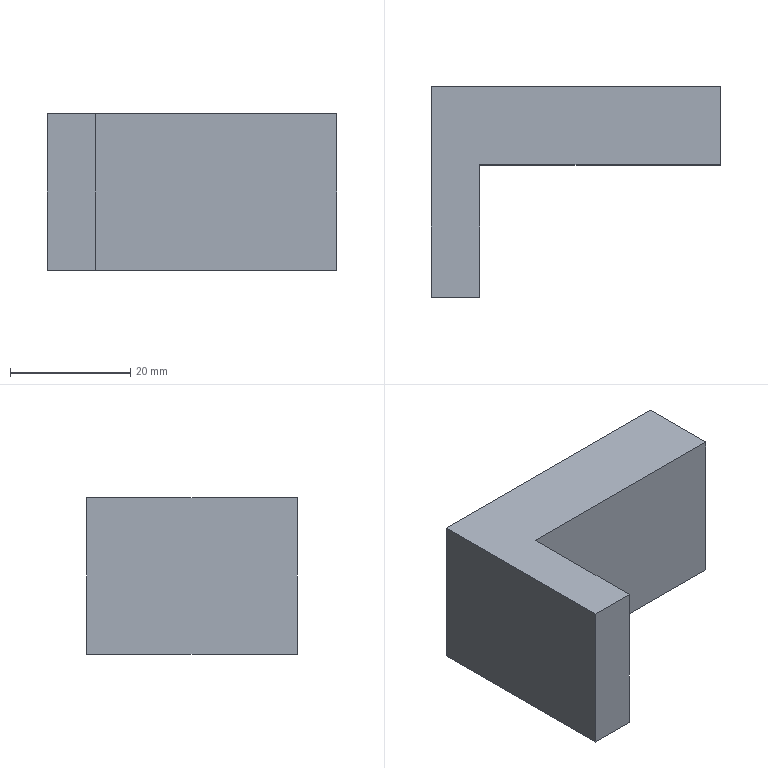Part | STEP file | 001-004-Feeding mechanism slider connecting plate | 1 solid | 8 faces | box 48 x 35 x 26 mm | volume 20800 mm3 | plane 8
STEP:
#1=CARTESIAN_POINT('',(0.,0.,0.));
#2=DIRECTION('',(0.,0.,1.));
#3=DIRECTION('',(1.,0.,0.));
#4=AXIS2_PLACEMENT_3D('',#1,#2,#3);
#5=CARTESIAN_POINT('',(24.,4.5,26.));
#6=VERTEX_POINT('',#5);
#7=CARTESIAN_POINT('',(24.,17.5,26.));
#8=VERTEX_POINT('',#7);
#9=CARTESIAN_POINT('',(24.,-17.5,26.));
#10=DIRECTION('',(0.,1.,0.));
#11=VECTOR('',#10,1.);
#12=LINE('',#9,#11);
#13=CARTESIAN_POINT('',(24.,-17.5,26.));
#14=DIRECTION('',(-1.,0.,0.));
#15=DIRECTION('',(0.,0.,1.));
#16=AXIS2_PLACEMENT_3D('',#13,#14,#15);
#17=PLANE('',#16);
#18=CARTESIAN_POINT('',(0.,0.));
#19=DIRECTION('',(0.,1.));
#20=VECTOR('',#19,1.);
#21=LINE('',#18,#20);
#22=(GEOMETRIC_REPRESENTATION_CONTEXT(2)PARAMETRIC_REPRESENTATION_CONTEXT()REPRESENTATION_CONTEXT('',''));
#23=DEFINITIONAL_REPRESENTATION('',(#21),#22);
#24=PCURVE('',#17,#23);
#25=CARTESIAN_POINT('',(0.,0.,26.));
#26=DIRECTION('',(0.,0.,-1.));
#27=DIRECTION('',(-1.,0.,0.));
#28=AXIS2_PLACEMENT_3D('',#25,#26,#27);
#29=PLANE('',#28);
#30=CARTESIAN_POINT('',(-24.,-17.5));
#31=DIRECTION('',(0.,1.));
#32=VECTOR('',#31,1.);
#33=LINE('',#30,#32);
#34=(GEOMETRIC_REPRESENTATION_CONTEXT(2)PARAMETRIC_REPRESENTATION_CONTEXT()REPRESENTATION_CONTEXT('',''));
#35=DEFINITIONAL_REPRESENTATION('',(#33),#34);
#36=PCURVE('',#29,#35);
#37=SURFACE_CURVE('',#12,(#24,#36),.PCURVE_S1.);
#38=EDGE_CURVE('',#6,#8,#37,.T.);
#39=ORIENTED_EDGE('',*,*,#38,.F.);
#40=CARTESIAN_POINT('',(24.,4.5,0.));
#41=VERTEX_POINT('',#40);
#42=CARTESIAN_POINT('',(24.,4.5,0.));
#43=DIRECTION('',(0.,0.,1.));
#44=VECTOR('',#43,1.);
#45=LINE('',#42,#44);
#46=CARTESIAN_POINT('',(-26.,22.));
#47=DIRECTION('',(1.,0.));
#48=VECTOR('',#47,1.);
#49=LINE('',#46,#48);
#50=(GEOMETRIC_REPRESENTATION_CONTEXT(2)PARAMETRIC_REPRESENTATION_CONTEXT()REPRESENTATION_CONTEXT('',''));
#51=DEFINITIONAL_REPRESENTATION('',(#49),#50);
#52=PCURVE('',#17,#51);
#53=CARTESIAN_POINT('',(24.,4.5,0.));
#54=DIRECTION('',(0.,1.,0.));
#55=DIRECTION('',(-1.,0.,0.));
#56=AXIS2_PLACEMENT_3D('',#53,#54,#55);
#57=PLANE('',#56);
#58=CARTESIAN_POINT('',(0.,0.));
#59=DIRECTION('',(0.,1.));
#60=VECTOR('',#59,1.);
#61=LINE('',#58,#60);
#62=(GEOMETRIC_REPRESENTATION_CONTEXT(2)PARAMETRIC_REPRESENTATION_CONTEXT()REPRESENTATION_CONTEXT('',''));
#63=DEFINITIONAL_REPRESENTATION('',(#61),#62);
#64=PCURVE('',#57,#63);
#65=SURFACE_CURVE('',#45,(#52,#64),.PCURVE_S1.);
#66=EDGE_CURVE('',#41,#6,#65,.T.);
#67=ORIENTED_EDGE('',*,*,#66,.F.);
#68=CARTESIAN_POINT('',(24.,17.5,0.));
#69=VERTEX_POINT('',#68);
#70=CARTESIAN_POINT('',(24.,-17.5,0.));
#71=DIRECTION('',(0.,1.,0.));
#72=VECTOR('',#71,1.);
#73=LINE('',#70,#72);
#74=CARTESIAN_POINT('',(-26.,0.));
#75=DIRECTION('',(0.,1.));
#76=VECTOR('',#75,1.);
#77=LINE('',#74,#76);
#78=(GEOMETRIC_REPRESENTATION_CONTEXT(2)PARAMETRIC_REPRESENTATION_CONTEXT()REPRESENTATION_CONTEXT('',''));
#79=DEFINITIONAL_REPRESENTATION('',(#77),#78);
#80=PCURVE('',#17,#79);
#81=CARTESIAN_POINT('',(0.,0.,0.));
#82=DIRECTION('',(0.,0.,-1.));
#83=DIRECTION('',(-1.,0.,0.));
#84=AXIS2_PLACEMENT_3D('',#81,#82,#83);
#85=PLANE('',#84);
#86=CARTESIAN_POINT('',(-24.,-17.5));
#87=DIRECTION('',(0.,1.));
#88=VECTOR('',#87,1.);
#89=LINE('',#86,#88);
#90=(GEOMETRIC_REPRESENTATION_CONTEXT(2)PARAMETRIC_REPRESENTATION_CONTEXT()REPRESENTATION_CONTEXT('',''));
#91=DEFINITIONAL_REPRESENTATION('',(#89),#90);
#92=PCURVE('',#85,#91);
#93=SURFACE_CURVE('',#73,(#80,#92),.PCURVE_S1.);
#94=EDGE_CURVE('',#41,#69,#93,.T.);
#95=ORIENTED_EDGE('',*,*,#94,.T.);
#96=CARTESIAN_POINT('',(24.,17.5,26.));
#97=DIRECTION('',(0.,0.,-1.));
#98=VECTOR('',#97,1.);
#99=LINE('',#96,#98);
#100=CARTESIAN_POINT('',(0.,35.));
#101=DIRECTION('',(-1.,0.));
#102=VECTOR('',#101,1.);
#103=LINE('',#100,#102);
#104=(GEOMETRIC_REPRESENTATION_CONTEXT(2)PARAMETRIC_REPRESENTATION_CONTEXT()REPRESENTATION_CONTEXT('',''));
#105=DEFINITIONAL_REPRESENTATION('',(#103),#104);
#106=PCURVE('',#17,#105);
#107=CARTESIAN_POINT('',(-24.,17.5,26.));
#108=DIRECTION('',(0.,-1.,0.));
#109=DIRECTION('',(0.,0.,-1.));
#110=AXIS2_PLACEMENT_3D('',#107,#108,#109);
#111=PLANE('',#110);
#112=CARTESIAN_POINT('',(0.,48.));
#113=DIRECTION('',(1.,0.));
#114=VECTOR('',#113,1.);
#115=LINE('',#112,#114);
#116=(GEOMETRIC_REPRESENTATION_CONTEXT(2)PARAMETRIC_REPRESENTATION_CONTEXT()REPRESENTATION_CONTEXT('',''));
#117=DEFINITIONAL_REPRESENTATION('',(#115),#116);
#118=PCURVE('',#111,#117);
#119=SURFACE_CURVE('',#99,(#106,#118),.PCURVE_S1.);
#120=EDGE_CURVE('',#8,#69,#119,.T.);
#121=ORIENTED_EDGE('',*,*,#120,.F.);
#122=EDGE_LOOP('',(#39,#67,#95,#121));
#123=FACE_BOUND('',#122,.T.);
#124=ADVANCED_FACE('',(#123),#17,.F.);
#125=CARTESIAN_POINT('',(-24.,17.5,0.));
#126=VERTEX_POINT('',#125);
#127=CARTESIAN_POINT('',(-24.,17.5,0.));
#128=DIRECTION('',(-1.,0.,0.));
#129=VECTOR('',#128,1.);
#130=LINE('',#127,#129);
#131=CARTESIAN_POINT('',(26.,0.));
#132=DIRECTION('',(0.,-1.));
#133=VECTOR('',#132,1.);
#134=LINE('',#131,#133);
#135=(GEOMETRIC_REPRESENTATION_CONTEXT(2)PARAMETRIC_REPRESENTATION_CONTEXT()REPRESENTATION_CONTEXT('',''));
#136=DEFINITIONAL_REPRESENTATION('',(#134),#135);
#137=PCURVE('',#111,#136);
#138=CARTESIAN_POINT('',(24.,17.5));
#139=DIRECTION('',(1.,0.));
#140=VECTOR('',#139,1.);
#141=LINE('',#138,#140);
#142=(GEOMETRIC_REPRESENTATION_CONTEXT(2)PARAMETRIC_REPRESENTATION_CONTEXT()REPRESENTATION_CONTEXT('',''));
#143=DEFINITIONAL_REPRESENTATION('',(#141),#142);
#144=PCURVE('',#85,#143);
#145=SURFACE_CURVE('',#130,(#137,#144),.PCURVE_S1.);
#146=EDGE_CURVE('',#69,#126,#145,.T.);
#147=ORIENTED_EDGE('',*,*,#146,.T.);
#148=CARTESIAN_POINT('',(-24.,17.5,26.));
#149=VERTEX_POINT('',#148);
#150=CARTESIAN_POINT('',(-24.,17.5,26.));
#151=DIRECTION('',(0.,0.,-1.));
#152=VECTOR('',#151,1.);
#153=LINE('',#150,#152);
#154=CARTESIAN_POINT('',(0.,0.));
#155=DIRECTION('',(1.,0.));
#156=VECTOR('',#155,1.);
#157=LINE('',#154,#156);
#158=(GEOMETRIC_REPRESENTATION_CONTEXT(2)PARAMETRIC_REPRESENTATION_CONTEXT()REPRESENTATION_CONTEXT('',''));
#159=DEFINITIONAL_REPRESENTATION('',(#157),#158);
#160=PCURVE('',#111,#159);
#161=CARTESIAN_POINT('',(-24.,-17.5,26.));
#162=DIRECTION('',(1.,0.,0.));
#163=DIRECTION('',(0.,0.,-1.));
#164=AXIS2_PLACEMENT_3D('',#161,#162,#163);
#165=PLANE('',#164);
#166=CARTESIAN_POINT('',(0.,35.));
#167=DIRECTION('',(1.,0.));
#168=VECTOR('',#167,1.);
#169=LINE('',#166,#168);
#170=(GEOMETRIC_REPRESENTATION_CONTEXT(2)PARAMETRIC_REPRESENTATION_CONTEXT()REPRESENTATION_CONTEXT('',''));
#171=DEFINITIONAL_REPRESENTATION('',(#169),#170);
#172=PCURVE('',#165,#171);
#173=SURFACE_CURVE('',#153,(#160,#172),.PCURVE_S1.);
#174=EDGE_CURVE('',#149,#126,#173,.T.);
#175=ORIENTED_EDGE('',*,*,#174,.F.);
#176=CARTESIAN_POINT('',(-24.,17.5,26.));
#177=DIRECTION('',(-1.,0.,0.));
#178=VECTOR('',#177,1.);
#179=LINE('',#176,#178);
#180=CARTESIAN_POINT('',(0.,0.));
#181=DIRECTION('',(0.,-1.));
#182=VECTOR('',#181,1.);
#183=LINE('',#180,#182);
#184=(GEOMETRIC_REPRESENTATION_CONTEXT(2)PARAMETRIC_REPRESENTATION_CONTEXT()REPRESENTATION_CONTEXT('',''));
#185=DEFINITIONAL_REPRESENTATION('',(#183),#184);
#186=PCURVE('',#111,#185);
#187=CARTESIAN_POINT('',(24.,17.5));
#188=DIRECTION('',(1.,0.));
#189=VECTOR('',#188,1.);
#190=LINE('',#187,#189);
#191=(GEOMETRIC_REPRESENTATION_CONTEXT(2)PARAMETRIC_REPRESENTATION_CONTEXT()REPRESENTATION_CONTEXT('',''));
#192=DEFINITIONAL_REPRESENTATION('',(#190),#191);
#193=PCURVE('',#29,#192);
#194=SURFACE_CURVE('',#179,(#186,#193),.PCURVE_S1.);
#195=EDGE_CURVE('',#8,#149,#194,.T.);
#196=ORIENTED_EDGE('',*,*,#195,.F.);
#197=ORIENTED_EDGE('',*,*,#120,.T.);
#198=EDGE_LOOP('',(#147,#175,#196,#197));
#199=FACE_BOUND('',#198,.T.);
#200=ADVANCED_FACE('',(#199),#111,.F.);
#201=CARTESIAN_POINT('',(-24.,-17.5,0.));
#202=VERTEX_POINT('',#201);
#203=CARTESIAN_POINT('',(-24.,-17.5,0.));
#204=DIRECTION('',(0.,-1.,0.));
#205=VECTOR('',#204,1.);
#206=LINE('',#203,#205);
#207=CARTESIAN_POINT('',(26.,0.));
#208=DIRECTION('',(0.,-1.));
#209=VECTOR('',#208,1.);
#210=LINE('',#207,#209);
#211=(GEOMETRIC_REPRESENTATION_CONTEXT(2)PARAMETRIC_REPRESENTATION_CONTEXT()REPRESENTATION_CONTEXT('',''));
#212=DEFINITIONAL_REPRESENTATION('',(#210),#211);
#213=PCURVE('',#165,#212);
#214=CARTESIAN_POINT('',(24.,-17.5));
#215=DIRECTION('',(0.,-1.));
#216=VECTOR('',#215,1.);
#217=LINE('',#214,#216);
#218=(GEOMETRIC_REPRESENTATION_CONTEXT(2)PARAMETRIC_REPRESENTATION_CONTEXT()REPRESENTATION_CONTEXT('',''));
#219=DEFINITIONAL_REPRESENTATION('',(#217),#218);
#220=PCURVE('',#85,#219);
#221=SURFACE_CURVE('',#206,(#213,#220),.PCURVE_S1.);
#222=EDGE_CURVE('',#126,#202,#221,.T.);
#223=ORIENTED_EDGE('',*,*,#222,.T.);
#224=CARTESIAN_POINT('',(-24.,-17.5,26.));
#225=VERTEX_POINT('',#224);
#226=CARTESIAN_POINT('',(-24.,-17.5,26.));
#227=DIRECTION('',(0.,0.,-1.));
#228=VECTOR('',#227,1.);
#229=LINE('',#226,#228);
#230=CARTESIAN_POINT('',(0.,0.));
#231=DIRECTION('',(1.,0.));
#232=VECTOR('',#231,1.);
#233=LINE('',#230,#232);
#234=(GEOMETRIC_REPRESENTATION_CONTEXT(2)PARAMETRIC_REPRESENTATION_CONTEXT()REPRESENTATION_CONTEXT('',''));
#235=DEFINITIONAL_REPRESENTATION('',(#233),#234);
#236=PCURVE('',#165,#235);
#237=CARTESIAN_POINT('',(-24.,-17.5,26.));
#238=DIRECTION('',(0.,1.,0.));
#239=DIRECTION('',(0.,0.,1.));
#240=AXIS2_PLACEMENT_3D('',#237,#238,#239);
#241=PLANE('',#240);
#242=CARTESIAN_POINT('',(0.,0.));
#243=DIRECTION('',(-1.,0.));
#244=VECTOR('',#243,1.);
#245=LINE('',#242,#244);
#246=(GEOMETRIC_REPRESENTATION_CONTEXT(2)PARAMETRIC_REPRESENTATION_CONTEXT()REPRESENTATION_CONTEXT('',''));
#247=DEFINITIONAL_REPRESENTATION('',(#245),#246);
#248=PCURVE('',#241,#247);
#249=SURFACE_CURVE('',#229,(#236,#248),.PCURVE_S1.);
#250=EDGE_CURVE('',#225,#202,#249,.T.);
#251=ORIENTED_EDGE('',*,*,#250,.F.);
#252=CARTESIAN_POINT('',(-24.,-17.5,26.));
#253=DIRECTION('',(0.,-1.,0.));
#254=VECTOR('',#253,1.);
#255=LINE('',#252,#254);
#256=CARTESIAN_POINT('',(0.,0.));
#257=DIRECTION('',(0.,-1.));
#258=VECTOR('',#257,1.);
#259=LINE('',#256,#258);
#260=(GEOMETRIC_REPRESENTATION_CONTEXT(2)PARAMETRIC_REPRESENTATION_CONTEXT()REPRESENTATION_CONTEXT('',''));
#261=DEFINITIONAL_REPRESENTATION('',(#259),#260);
#262=PCURVE('',#165,#261);
#263=CARTESIAN_POINT('',(24.,-17.5));
#264=DIRECTION('',(0.,-1.));
#265=VECTOR('',#264,1.);
#266=LINE('',#263,#265);
#267=(GEOMETRIC_REPRESENTATION_CONTEXT(2)PARAMETRIC_REPRESENTATION_CONTEXT()REPRESENTATION_CONTEXT('',''));
#268=DEFINITIONAL_REPRESENTATION('',(#266),#267);
#269=PCURVE('',#29,#268);
#270=SURFACE_CURVE('',#255,(#262,#269),.PCURVE_S1.);
#271=EDGE_CURVE('',#149,#225,#270,.T.);
#272=ORIENTED_EDGE('',*,*,#271,.F.);
#273=ORIENTED_EDGE('',*,*,#174,.T.);
#274=EDGE_LOOP('',(#223,#251,#272,#273));
#275=FACE_BOUND('',#274,.T.);
#276=ADVANCED_FACE('',(#275),#165,.F.);
#277=CARTESIAN_POINT('',(-16.,-17.5,0.));
#278=VERTEX_POINT('',#277);
#279=CARTESIAN_POINT('',(-24.,-17.5,0.));
#280=DIRECTION('',(1.,0.,0.));
#281=VECTOR('',#280,1.);
#282=LINE('',#279,#281);
#283=CARTESIAN_POINT('',(-26.,0.));
#284=DIRECTION('',(0.,1.));
#285=VECTOR('',#284,1.);
#286=LINE('',#283,#285);
#287=(GEOMETRIC_REPRESENTATION_CONTEXT(2)PARAMETRIC_REPRESENTATION_CONTEXT()REPRESENTATION_CONTEXT('',''));
#288=DEFINITIONAL_REPRESENTATION('',(#286),#287);
#289=PCURVE('',#241,#288);
#290=CARTESIAN_POINT('',(24.,-17.5));
#291=DIRECTION('',(-1.,0.));
#292=VECTOR('',#291,1.);
#293=LINE('',#290,#292);
#294=(GEOMETRIC_REPRESENTATION_CONTEXT(2)PARAMETRIC_REPRESENTATION_CONTEXT()REPRESENTATION_CONTEXT('',''));
#295=DEFINITIONAL_REPRESENTATION('',(#293),#294);
#296=PCURVE('',#85,#295);
#297=SURFACE_CURVE('',#282,(#289,#296),.PCURVE_S1.);
#298=EDGE_CURVE('',#202,#278,#297,.T.);
#299=ORIENTED_EDGE('',*,*,#298,.T.);
#300=CARTESIAN_POINT('',(-16.,-17.5,26.));
#301=VERTEX_POINT('',#300);
#302=CARTESIAN_POINT('',(-16.,-17.5,0.));
#303=DIRECTION('',(0.,0.,1.));
#304=VECTOR('',#303,1.);
#305=LINE('',#302,#304);
#306=CARTESIAN_POINT('',(-26.,8.));
#307=DIRECTION('',(1.,0.));
#308=VECTOR('',#307,1.);
#309=LINE('',#306,#308);
#310=(GEOMETRIC_REPRESENTATION_CONTEXT(2)PARAMETRIC_REPRESENTATION_CONTEXT()REPRESENTATION_CONTEXT('',''));
#311=DEFINITIONAL_REPRESENTATION('',(#309),#310);
#312=PCURVE('',#241,#311);
#313=CARTESIAN_POINT('',(-16.,-17.5,0.));
#314=DIRECTION('',(-1.,0.,0.));
#315=DIRECTION('',(0.,0.,1.));
#316=AXIS2_PLACEMENT_3D('',#313,#314,#315);
#317=PLANE('',#316);
#318=CARTESIAN_POINT('',(0.,0.));
#319=DIRECTION('',(1.,0.));
#320=VECTOR('',#319,1.);
#321=LINE('',#318,#320);
#322=(GEOMETRIC_REPRESENTATION_CONTEXT(2)PARAMETRIC_REPRESENTATION_CONTEXT()REPRESENTATION_CONTEXT('',''));
#323=DEFINITIONAL_REPRESENTATION('',(#321),#322);
#324=PCURVE('',#317,#323);
#325=SURFACE_CURVE('',#305,(#312,#324),.PCURVE_S1.);
#326=EDGE_CURVE('',#278,#301,#325,.T.);
#327=ORIENTED_EDGE('',*,*,#326,.T.);
#328=CARTESIAN_POINT('',(-24.,-17.5,26.));
#329=DIRECTION('',(1.,0.,0.));
#330=VECTOR('',#329,1.);
#331=LINE('',#328,#330);
#332=CARTESIAN_POINT('',(0.,0.));
#333=DIRECTION('',(0.,1.));
#334=VECTOR('',#333,1.);
#335=LINE('',#332,#334);
#336=(GEOMETRIC_REPRESENTATION_CONTEXT(2)PARAMETRIC_REPRESENTATION_CONTEXT()REPRESENTATION_CONTEXT('',''));
#337=DEFINITIONAL_REPRESENTATION('',(#335),#336);
#338=PCURVE('',#241,#337);
#339=CARTESIAN_POINT('',(24.,-17.5));
#340=DIRECTION('',(-1.,0.));
#341=VECTOR('',#340,1.);
#342=LINE('',#339,#341);
#343=(GEOMETRIC_REPRESENTATION_CONTEXT(2)PARAMETRIC_REPRESENTATION_CONTEXT()REPRESENTATION_CONTEXT('',''));
#344=DEFINITIONAL_REPRESENTATION('',(#342),#343);
#345=PCURVE('',#29,#344);
#346=SURFACE_CURVE('',#331,(#338,#345),.PCURVE_S1.);
#347=EDGE_CURVE('',#225,#301,#346,.T.);
#348=ORIENTED_EDGE('',*,*,#347,.F.);
#349=ORIENTED_EDGE('',*,*,#250,.T.);
#350=EDGE_LOOP('',(#299,#327,#348,#349));
#351=FACE_BOUND('',#350,.T.);
#352=ADVANCED_FACE('',(#351),#241,.F.);
#353=ORIENTED_EDGE('',*,*,#347,.T.);
#354=CARTESIAN_POINT('',(-16.,4.5,26.));
#355=VERTEX_POINT('',#354);
#356=CARTESIAN_POINT('',(-16.,-17.5,26.));
#357=DIRECTION('',(0.,-1.,0.));
#358=VECTOR('',#357,1.);
#359=LINE('',#356,#358);
#360=CARTESIAN_POINT('',(16.,-17.5));
#361=DIRECTION('',(0.,-1.));
#362=VECTOR('',#361,1.);
#363=LINE('',#360,#362);
#364=(GEOMETRIC_REPRESENTATION_CONTEXT(2)PARAMETRIC_REPRESENTATION_CONTEXT()REPRESENTATION_CONTEXT('',''));
#365=DEFINITIONAL_REPRESENTATION('',(#363),#364);
#366=PCURVE('',#29,#365);
#367=CARTESIAN_POINT('',(26.,0.));
#368=DIRECTION('',(0.,-1.));
#369=VECTOR('',#368,1.);
#370=LINE('',#367,#369);
#371=(GEOMETRIC_REPRESENTATION_CONTEXT(2)PARAMETRIC_REPRESENTATION_CONTEXT()REPRESENTATION_CONTEXT('',''));
#372=DEFINITIONAL_REPRESENTATION('',(#370),#371);
#373=PCURVE('',#317,#372);
#374=SURFACE_CURVE('',#359,(#366,#373),.PCURVE_S1.);
#375=EDGE_CURVE('',#355,#301,#374,.T.);
#376=ORIENTED_EDGE('',*,*,#375,.F.);
#377=CARTESIAN_POINT('',(24.,4.5,26.));
#378=DIRECTION('',(-1.,0.,0.));
#379=VECTOR('',#378,1.);
#380=LINE('',#377,#379);
#381=CARTESIAN_POINT('',(-24.,4.5));
#382=DIRECTION('',(1.,0.));
#383=VECTOR('',#382,1.);
#384=LINE('',#381,#383);
#385=(GEOMETRIC_REPRESENTATION_CONTEXT(2)PARAMETRIC_REPRESENTATION_CONTEXT()REPRESENTATION_CONTEXT('',''));
#386=DEFINITIONAL_REPRESENTATION('',(#384),#385);
#387=PCURVE('',#29,#386);
#388=CARTESIAN_POINT('',(0.,26.));
#389=DIRECTION('',(1.,0.));
#390=VECTOR('',#389,1.);
#391=LINE('',#388,#390);
#392=(GEOMETRIC_REPRESENTATION_CONTEXT(2)PARAMETRIC_REPRESENTATION_CONTEXT()REPRESENTATION_CONTEXT('',''));
#393=DEFINITIONAL_REPRESENTATION('',(#391),#392);
#394=PCURVE('',#57,#393);
#395=SURFACE_CURVE('',#380,(#387,#394),.PCURVE_S1.);
#396=EDGE_CURVE('',#6,#355,#395,.T.);
#397=ORIENTED_EDGE('',*,*,#396,.F.);
#398=ORIENTED_EDGE('',*,*,#38,.T.);
#399=ORIENTED_EDGE('',*,*,#195,.T.);
#400=ORIENTED_EDGE('',*,*,#271,.T.);
#401=EDGE_LOOP('',(#353,#376,#397,#398,#399,#400));
#402=FACE_BOUND('',#401,.T.);
#403=ADVANCED_FACE('',(#402),#29,.F.);
#404=CARTESIAN_POINT('',(-16.,4.5,0.));
#405=VERTEX_POINT('',#404);
#406=CARTESIAN_POINT('',(-16.,-17.5,0.));
#407=DIRECTION('',(0.,-1.,0.));
#408=VECTOR('',#407,1.);
#409=LINE('',#406,#408);
#410=CARTESIAN_POINT('',(16.,-17.5));
#411=DIRECTION('',(0.,-1.));
#412=VECTOR('',#411,1.);
#413=LINE('',#410,#412);
#414=(GEOMETRIC_REPRESENTATION_CONTEXT(2)PARAMETRIC_REPRESENTATION_CONTEXT()REPRESENTATION_CONTEXT('',''));
#415=DEFINITIONAL_REPRESENTATION('',(#413),#414);
#416=PCURVE('',#85,#415);
#417=CARTESIAN_POINT('',(0.,0.));
#418=DIRECTION('',(0.,-1.));
#419=VECTOR('',#418,1.);
#420=LINE('',#417,#419);
#421=(GEOMETRIC_REPRESENTATION_CONTEXT(2)PARAMETRIC_REPRESENTATION_CONTEXT()REPRESENTATION_CONTEXT('',''));
#422=DEFINITIONAL_REPRESENTATION('',(#420),#421);
#423=PCURVE('',#317,#422);
#424=SURFACE_CURVE('',#409,(#416,#423),.PCURVE_S1.);
#425=EDGE_CURVE('',#405,#278,#424,.T.);
#426=ORIENTED_EDGE('',*,*,#425,.T.);
#427=ORIENTED_EDGE('',*,*,#298,.F.);
#428=ORIENTED_EDGE('',*,*,#222,.F.);
#429=ORIENTED_EDGE('',*,*,#146,.F.);
#430=ORIENTED_EDGE('',*,*,#94,.F.);
#431=CARTESIAN_POINT('',(24.,4.5,0.));
#432=DIRECTION('',(-1.,0.,0.));
#433=VECTOR('',#432,1.);
#434=LINE('',#431,#433);
#435=CARTESIAN_POINT('',(-24.,4.5));
#436=DIRECTION('',(1.,0.));
#437=VECTOR('',#436,1.);
#438=LINE('',#435,#437);
#439=(GEOMETRIC_REPRESENTATION_CONTEXT(2)PARAMETRIC_REPRESENTATION_CONTEXT()REPRESENTATION_CONTEXT('',''));
#440=DEFINITIONAL_REPRESENTATION('',(#438),#439);
#441=PCURVE('',#85,#440);
#442=CARTESIAN_POINT('',(0.,0.));
#443=DIRECTION('',(1.,0.));
#444=VECTOR('',#443,1.);
#445=LINE('',#442,#444);
#446=(GEOMETRIC_REPRESENTATION_CONTEXT(2)PARAMETRIC_REPRESENTATION_CONTEXT()REPRESENTATION_CONTEXT('',''));
#447=DEFINITIONAL_REPRESENTATION('',(#445),#446);
#448=PCURVE('',#57,#447);
#449=SURFACE_CURVE('',#434,(#441,#448),.PCURVE_S1.);
#450=EDGE_CURVE('',#41,#405,#449,.T.);
#451=ORIENTED_EDGE('',*,*,#450,.T.);
#452=EDGE_LOOP('',(#426,#427,#428,#429,#430,#451));
#453=FACE_BOUND('',#452,.T.);
#454=ADVANCED_FACE('',(#453),#85,.T.);
#455=ORIENTED_EDGE('',*,*,#375,.T.);
#456=ORIENTED_EDGE('',*,*,#326,.F.);
#457=ORIENTED_EDGE('',*,*,#425,.F.);
#458=CARTESIAN_POINT('',(-16.,4.5,0.));
#459=DIRECTION('',(0.,0.,1.));
#460=VECTOR('',#459,1.);
#461=LINE('',#458,#460);
#462=CARTESIAN_POINT('',(0.,22.));
#463=DIRECTION('',(1.,0.));
#464=VECTOR('',#463,1.);
#465=LINE('',#462,#464);
#466=(GEOMETRIC_REPRESENTATION_CONTEXT(2)PARAMETRIC_REPRESENTATION_CONTEXT()REPRESENTATION_CONTEXT('',''));
#467=DEFINITIONAL_REPRESENTATION('',(#465),#466);
#468=PCURVE('',#317,#467);
#469=CARTESIAN_POINT('',(40.,0.));
#470=DIRECTION('',(0.,1.));
#471=VECTOR('',#470,1.);
#472=LINE('',#469,#471);
#473=(GEOMETRIC_REPRESENTATION_CONTEXT(2)PARAMETRIC_REPRESENTATION_CONTEXT()REPRESENTATION_CONTEXT('',''));
#474=DEFINITIONAL_REPRESENTATION('',(#472),#473);
#475=PCURVE('',#57,#474);
#476=SURFACE_CURVE('',#461,(#468,#475),.PCURVE_S1.);
#477=EDGE_CURVE('',#405,#355,#476,.T.);
#478=ORIENTED_EDGE('',*,*,#477,.T.);
#479=EDGE_LOOP('',(#455,#456,#457,#478));
#480=FACE_BOUND('',#479,.T.);
#481=ADVANCED_FACE('',(#480),#317,.F.);
#482=ORIENTED_EDGE('',*,*,#396,.T.);
#483=ORIENTED_EDGE('',*,*,#477,.F.);
#484=ORIENTED_EDGE('',*,*,#450,.F.);
#485=ORIENTED_EDGE('',*,*,#66,.T.);
#486=EDGE_LOOP('',(#482,#483,#484,#485));
#487=FACE_BOUND('',#486,.T.);
#488=ADVANCED_FACE('',(#487),#57,.F.);
#489=CLOSED_SHELL('',(#124,#200,#276,#352,#403,#454,#481,#488));
#490=MANIFOLD_SOLID_BREP('',#489);
#491=(LENGTH_UNIT()NAMED_UNIT(*)SI_UNIT(.MILLI.,.METRE.));
#492=UNCERTAINTY_MEASURE_WITH_UNIT(LENGTH_MEASURE(0.0000001),#491,'','');
#493=(NAMED_UNIT(*)PLANE_ANGLE_UNIT()SI_UNIT($,.RADIAN.));
#494=(NAMED_UNIT(*)SI_UNIT($,.STERADIAN.)SOLID_ANGLE_UNIT());
#495=(GEOMETRIC_REPRESENTATION_CONTEXT(3)GLOBAL_UNCERTAINTY_ASSIGNED_CONTEXT((#492))GLOBAL_UNIT_ASSIGNED_CONTEXT((#491,#493,#494))REPRESENTATION_CONTEXT('',''));
#496=ADVANCED_BREP_SHAPE_REPRESENTATION('',(#4,#490),#495);